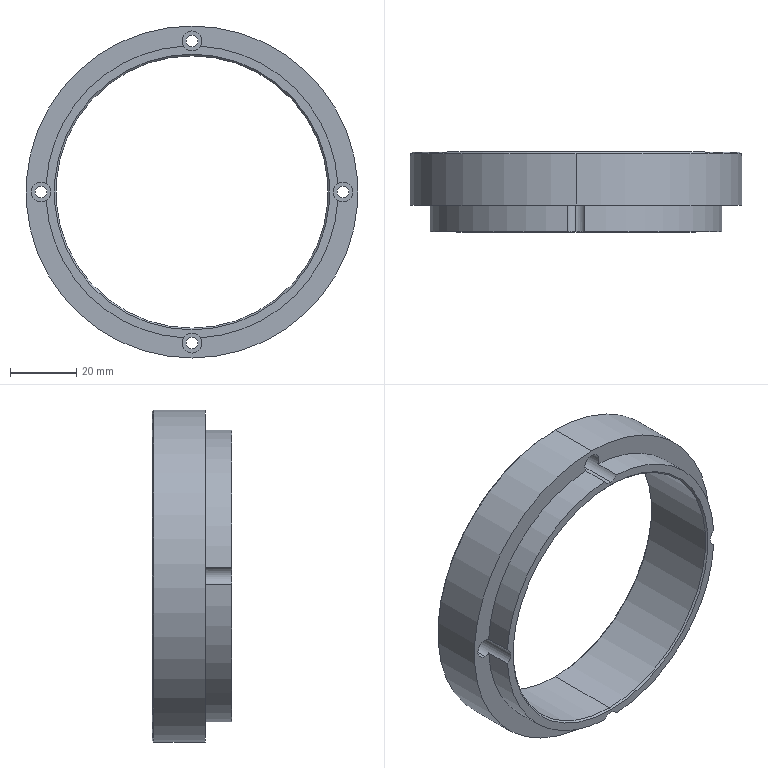Part | STEP file | ND25021-01-JDKM-02-SL | 1 solid | 37 faces | box 100 x 24 x 100 mm | volume 46236 mm3 | cylinder 24 | plane 7 | cone 6 | commonest cylinder face diameters 3.5 x8 6 x8 88 x4 82 x2 100 x2